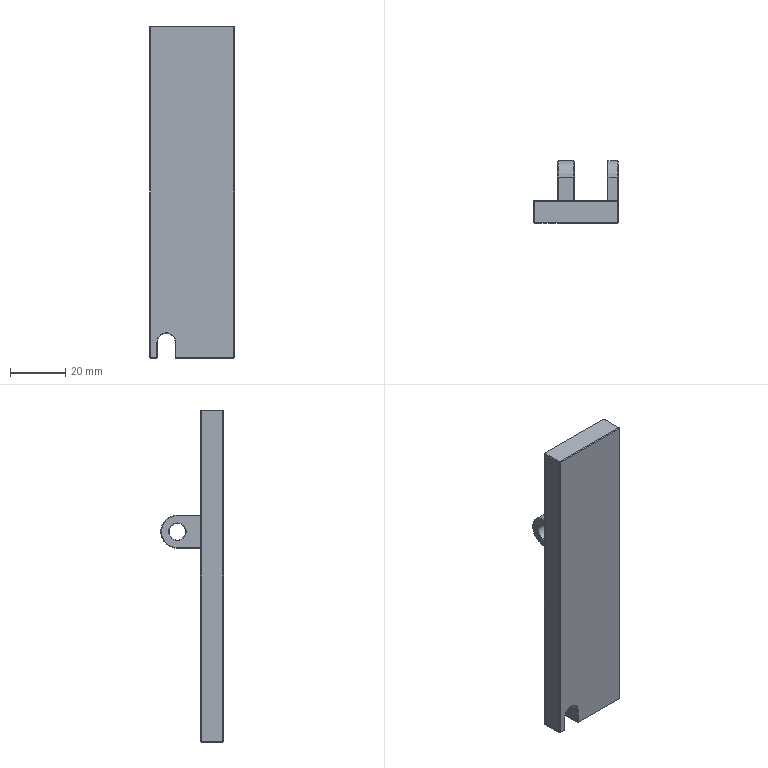Part | STEP file | 2008 | 1 solid | 68 faces | box 30.6 x 22.5 x 120 mm | volume 30242 mm3 | plane 45 | cone 15 | cylinder 8 | commonest cylinder face diameters 6 x4 6.4 x2 12 x2